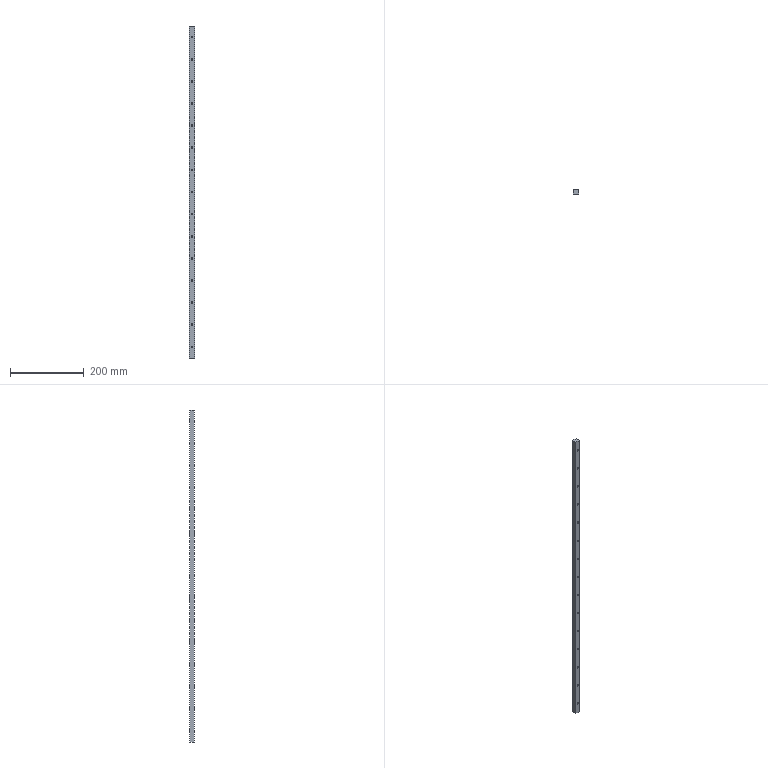Part | SolidWorks | features ICE 2, Extrusion 1, LPattern 1 | 1 solid | 81 faces | box 15 x 12.5 x 900 mm | volume 164933 mm3 | cylinder 60 | plane 21 | commonest cylinder face diameters 4.5 x30 6 x30